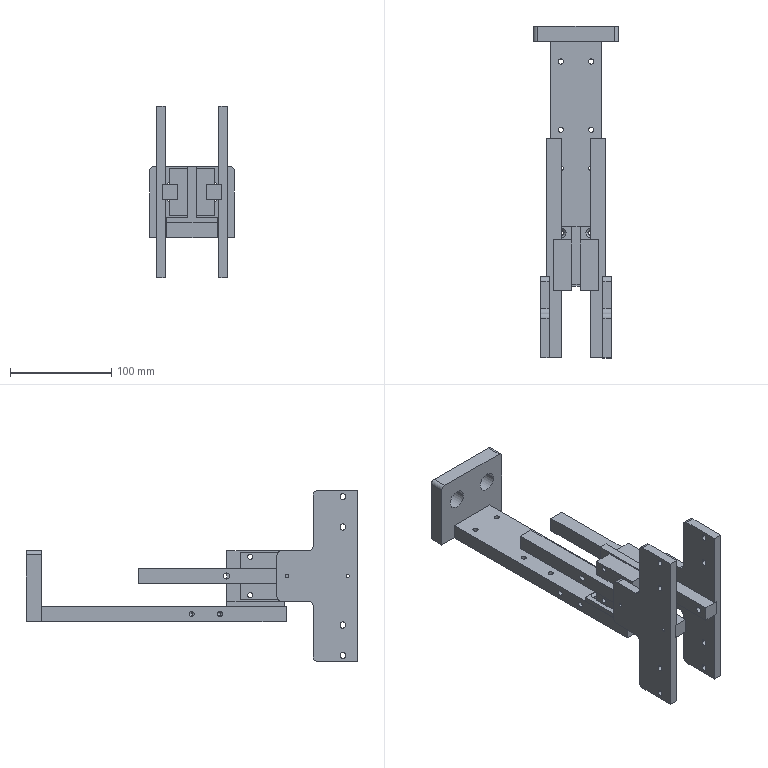Part | 9 solids | 256 faces | box 84 x 328 x 170 mm | volume 602327 mm3 | cylinder 134 | plane 98 | cone 24 | commonest cylinder face diameters 5 x52 5.2 x24 6 x12 10 x12 3.3 x8 5.5 x8